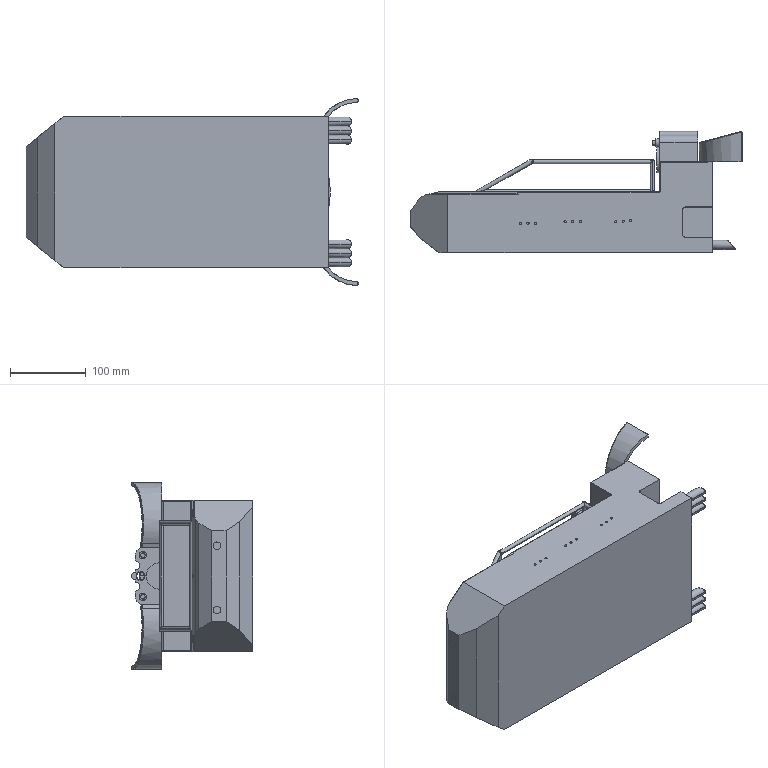Part | SolidWorks | features ICE 37, Fillet 7, Chamfer 2, 3DProfileFeature 1, BossThin 1, Extrusion 1, MirrorPattern 1, Shell 1, WeldMemberFeat 1, WeldmentFeature 1 | 22 solids | 336 faces | box 438.814 x 160 x 247.251 mm | volume 4513172 mm3 | cylinder 159 | plane 155 | spline 10 | cone 4 | torus 4 | sphere 4 | commonest cylinder face diameters 5.5 x38 3 x36 10 x24 2 x17 12 x16 4 x8